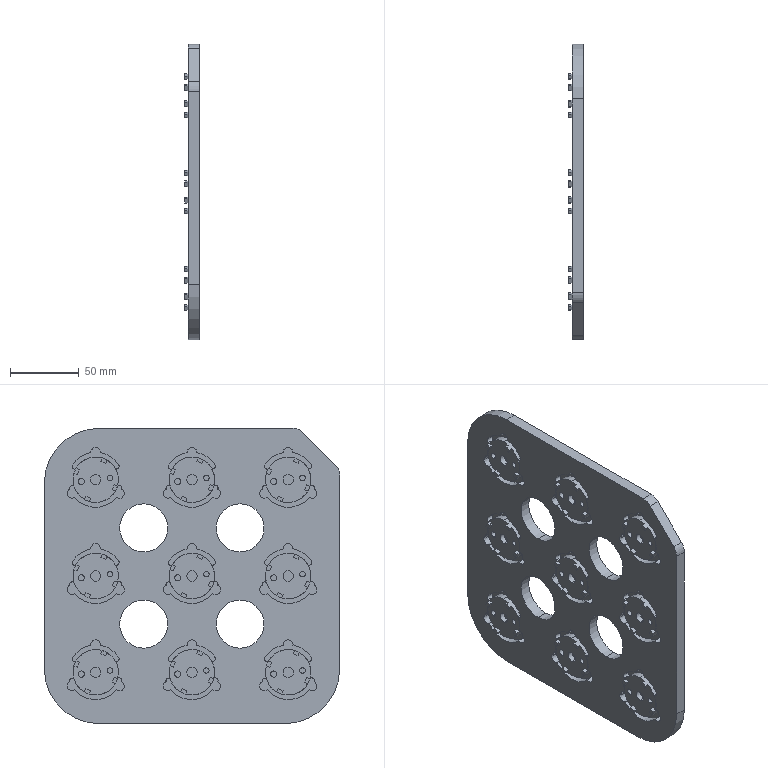Part | SolidWorks | features ICE 6, MoveCopyBody 6, Cut 3, Fillet 3, Chamfer 1, Extrusion 1, LPattern 1, MoveFace 1, Stock 1 | 1 solid | 488 faces | box 10.7 x 214.9 x 214.8 mm | volume 309606 mm3 | cylinder 274 | plane 214 | commonest cylinder face diameters 4 x117 7 x54 40 x36 4.5 x18 7.5 x18 33 x18